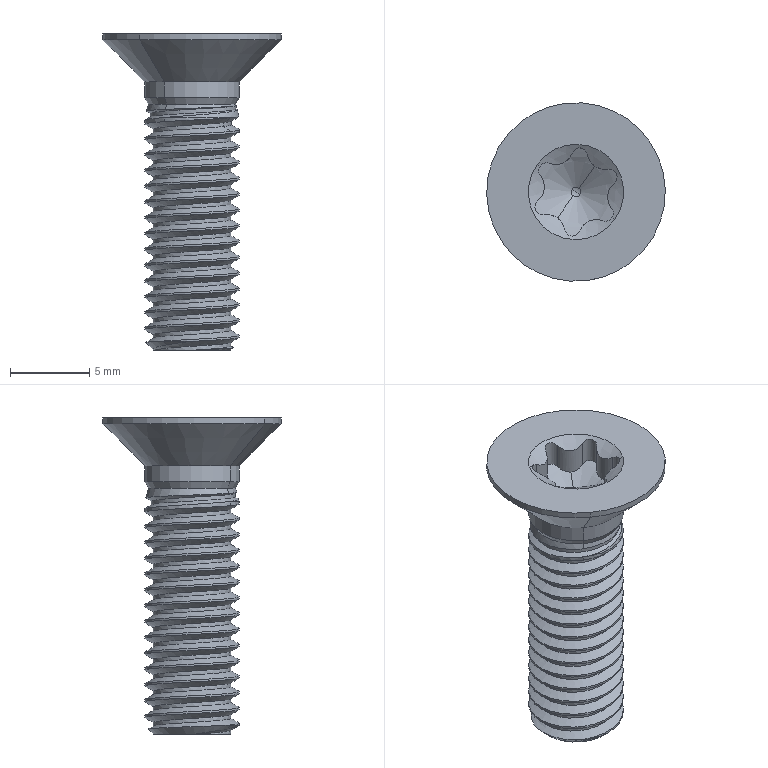Part | SolidWorks | features BaseBody 1 | 1 solid | 76 faces | box 11.3 x 11.3 x 20 mm | volume 545.688 mm3 | cylinder 52 | cone 14 | spline 6 | plane 2 | sphere 2 | commonest cylinder face diameters 6 x33 1.01 x9 2.274 x8 11.3 x2